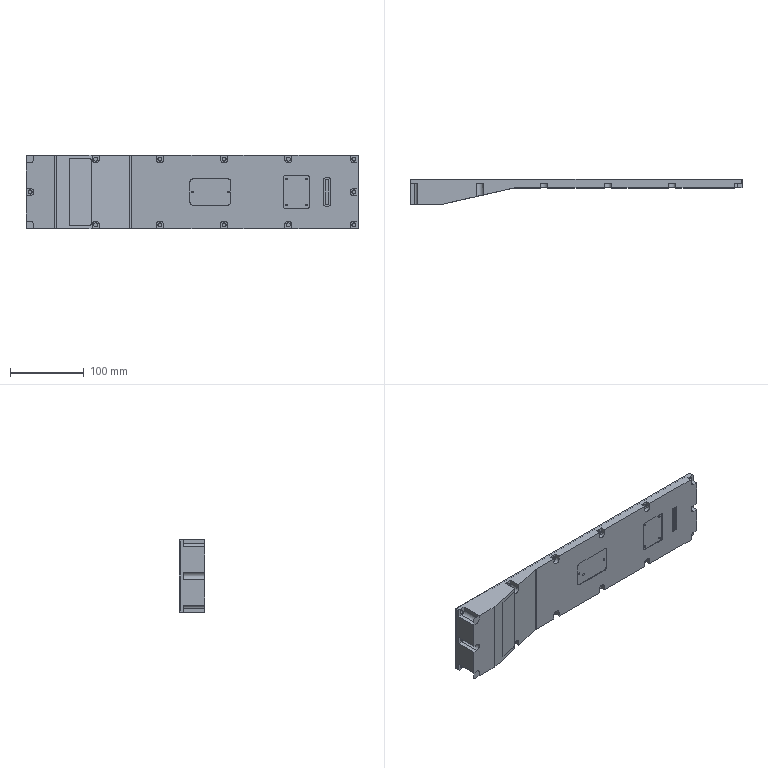NC program | Mastercam | posted with a generic post | part box 450 x 35 x 100 mm
Lines 1 to 35 of 140701:
%
:0001()
(MATERIAL - ALUMINUM MM - 2024)
(T24|100 FEM |H24|XY STOCK TO LEAVE - 0.|Z STOCK TO LEAVE - .2)
(T12|12 FEM |H12|XY STOCK TO LEAVE - .5|Z STOCK TO LEAVE - 0.)
(T20|20 FEM |H20)
(T7|6 CHM |H7)
(T8|8 FEM |H8|XY STOCK TO LEAVE - .1|Z STOCK TO LEAVE - .1)
(T6|6 FEM |H6|XY STOCK TO LEAVE - .1|Z STOCK TO LEAVE - .1)
(T4|4 FEM |H4|XY STOCK TO LEAVE - .05|Z STOCK TO LEAVE - .1)
(T11|10 BNOS |H11)
(T13|12 FEM |H13)
(T1|4 BM/BNOS |H1)
(T2|3 FEM |H2|XY STOCK TO LEAVE - -.01|Z STOCK TO LEAVE - 0.)
N100 G21
N102 G0 G17 G40 G80 G90 G94 G98
N104 G0 G28 G91 Z0.
N106 G0 G28 X0. Y0.
(100 FEM |TOOL - 24|DIA. OFF. - 24|LEN. - 24|TOOL DIA. - 100.)
N108 T24 M6
N110 G0 G54 G90 X-339. Y22.498 C0. B0. S4000 M3
N112 G43 H24 Z50.2
N114 Z2.2
N116 G1 Z.2 F600.
N118 X279. F1000.
N120 G2 X301.498 Y0. J-22.498
N122 X279. Y-22.498 I-22.498
N124 G1 X-339.
N126 G0 Z50.2
N128 M5
N130 G0 G28 G91 Z0.
N132 G28
N134 M01
N136 G0 G17 G40 G80 G90 G94 G98
N138 G0 G28 G91 Z0.